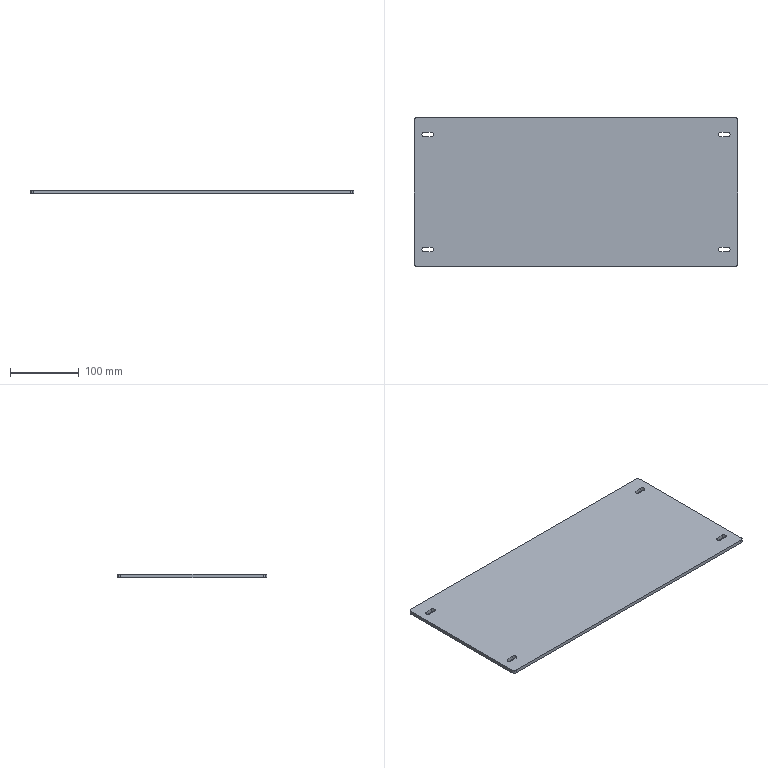Part | STEP file | DCV-000-010 | 1 solid | 30 faces | box 470 x 217 x 5 mm | volume 507673 mm3 | cylinder 16 | plane 14 | commonest cylinder face diameters 7 x8 10 x8